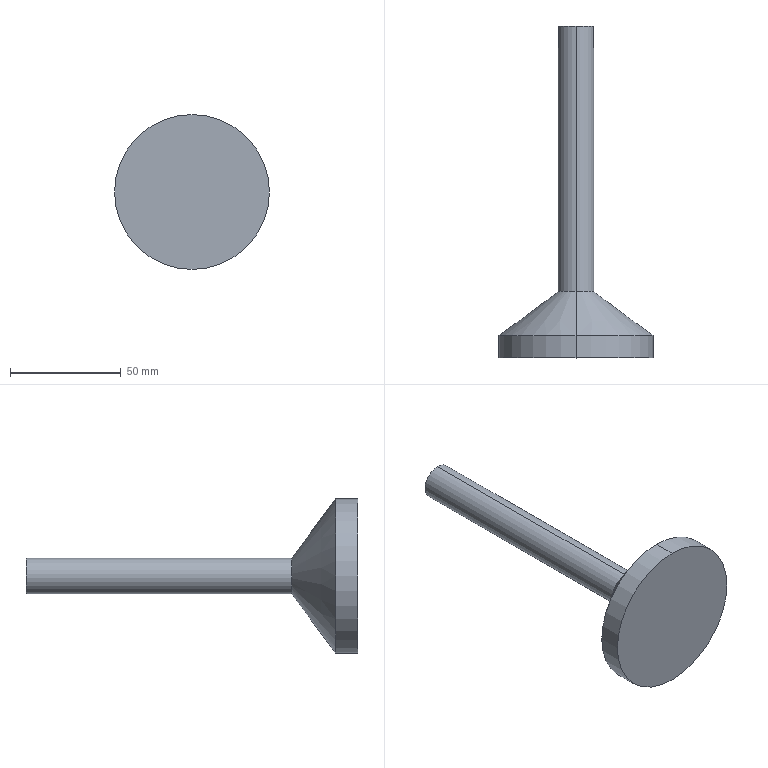Part | SolidWorks | features BaseBody 1 | 1 solid | 8 faces | box 70 x 150 x 70 mm | volume 95473 mm3 | cylinder 4 | cone 2 | plane 2 | commonest cylinder face diameters 16 x2 70 x2
STEP:
#1=CARTESIAN_POINT('',(0.,0.,-35.));
#2=VERTEX_POINT('',#1);
#3=CARTESIAN_POINT('',(0.,0.,35.));
#4=VERTEX_POINT('',#3);
#5=CARTESIAN_POINT('',(0.,0.,0.));
#6=DIRECTION('',(0.,-1.,0.));
#7=DIRECTION('',(0.,0.,1.));
#8=AXIS2_PLACEMENT_3D('',#5,#6,#7);
#9=CIRCLE('',#8,35.);
#10=EDGE_CURVE('',#2,#4,#9,.T.);
#11=ORIENTED_EDGE('',*,*,#10,.F.);
#12=CARTESIAN_POINT('',(0.,10.,-35.));
#13=VERTEX_POINT('',#12);
#14=CARTESIAN_POINT('',(0.,150.,-35.));
#15=DIRECTION('',(0.,1.,0.));
#16=VECTOR('',#15,1000.);
#17=LINE('',#14,#16);
#18=EDGE_CURVE('',#2,#13,#17,.T.);
#19=ORIENTED_EDGE('',*,*,#18,.T.);
#20=CARTESIAN_POINT('',(0.,10.,35.));
#21=VERTEX_POINT('',#20);
#22=CARTESIAN_POINT('',(0.,10.,0.));
#23=DIRECTION('',(0.,-1.,0.));
#24=DIRECTION('',(0.,0.,1.));
#25=AXIS2_PLACEMENT_3D('',#22,#23,#24);
#26=CIRCLE('',#25,35.);
#27=EDGE_CURVE('',#13,#21,#26,.T.);
#28=ORIENTED_EDGE('',*,*,#27,.T.);
#29=CARTESIAN_POINT('',(0.,150.,35.));
#30=DIRECTION('',(0.,1.,0.));
#31=VECTOR('',#30,1000.);
#32=LINE('',#29,#31);
#33=EDGE_CURVE('',#4,#21,#32,.T.);
#34=ORIENTED_EDGE('',*,*,#33,.F.);
#35=EDGE_LOOP('',(#11,#19,#28,#34));
#36=FACE_OUTER_BOUND('',#35,.T.);
#37=CARTESIAN_POINT('',(0.,150.,0.));
#38=DIRECTION('',(0.,1.,0.));
#39=DIRECTION('',(0.,0.,1.));
#40=AXIS2_PLACEMENT_3D('',#37,#38,#39);
#41=CYLINDRICAL_SURFACE('',#40,35.);
#42=ADVANCED_FACE('',(#36),#41,.T.);
#43=CARTESIAN_POINT('',(0.,30.,-8.));
#44=VERTEX_POINT('',#43);
#45=CARTESIAN_POINT('',(0.,30.,8.));
#46=VERTEX_POINT('',#45);
#47=CARTESIAN_POINT('',(0.,30.,0.));
#48=DIRECTION('',(0.,-1.,0.));
#49=DIRECTION('',(0.,0.,-1.));
#50=AXIS2_PLACEMENT_3D('',#47,#48,#49);
#51=CIRCLE('',#50,8.);
#52=EDGE_CURVE('',#44,#46,#51,.T.);
#53=ORIENTED_EDGE('',*,*,#52,.T.);
#54=CARTESIAN_POINT('',(0.,10.,35.));
#55=DIRECTION('',(0.,-0.5952,0.8036));
#56=VECTOR('',#55,1000.);
#57=LINE('',#54,#56);
#58=EDGE_CURVE('',#46,#21,#57,.T.);
#59=ORIENTED_EDGE('',*,*,#58,.T.);
#60=ORIENTED_EDGE('',*,*,#27,.F.);
#61=CARTESIAN_POINT('',(0.,10.,-35.));
#62=DIRECTION('',(0.,-0.5952,-0.8036));
#63=VECTOR('',#62,1000.);
#64=LINE('',#61,#63);
#65=EDGE_CURVE('',#44,#13,#64,.T.);
#66=ORIENTED_EDGE('',*,*,#65,.F.);
#67=EDGE_LOOP('',(#53,#59,#60,#66));
#68=FACE_OUTER_BOUND('',#67,.T.);
#69=CARTESIAN_POINT('',(0.,10.,0.));
#70=DIRECTION('',(0.,-1.,0.));
#71=DIRECTION('',(0.,0.,-1.));
#72=AXIS2_PLACEMENT_3D('',#69,#70,#71);
#73=CONICAL_SURFACE('',#72,35.,0.9332);
#74=ADVANCED_FACE('',(#68),#73,.T.);
#75=ORIENTED_EDGE('',*,*,#52,.F.);
#76=CARTESIAN_POINT('',(0.,150.,-8.));
#77=VERTEX_POINT('',#76);
#78=CARTESIAN_POINT('',(0.,150.,-8.));
#79=DIRECTION('',(0.,1.,0.));
#80=VECTOR('',#79,1000.);
#81=LINE('',#78,#80);
#82=EDGE_CURVE('',#44,#77,#81,.T.);
#83=ORIENTED_EDGE('',*,*,#82,.T.);
#84=CARTESIAN_POINT('',(0.,150.,8.));
#85=VERTEX_POINT('',#84);
#86=CARTESIAN_POINT('',(0.,150.,0.));
#87=DIRECTION('',(0.,-1.,0.));
#88=DIRECTION('',(0.,0.,1.));
#89=AXIS2_PLACEMENT_3D('',#86,#87,#88);
#90=CIRCLE('',#89,8.);
#91=EDGE_CURVE('',#77,#85,#90,.T.);
#92=ORIENTED_EDGE('',*,*,#91,.T.);
#93=CARTESIAN_POINT('',(0.,150.,8.));
#94=DIRECTION('',(0.,1.,0.));
#95=VECTOR('',#94,1000.);
#96=LINE('',#93,#95);
#97=EDGE_CURVE('',#46,#85,#96,.T.);
#98=ORIENTED_EDGE('',*,*,#97,.F.);
#99=EDGE_LOOP('',(#75,#83,#92,#98));
#100=FACE_OUTER_BOUND('',#99,.T.);
#101=CARTESIAN_POINT('',(0.,150.,0.));
#102=DIRECTION('',(0.,1.,0.));
#103=DIRECTION('',(0.,0.,1.));
#104=AXIS2_PLACEMENT_3D('',#101,#102,#103);
#105=CYLINDRICAL_SURFACE('',#104,8.);
#106=ADVANCED_FACE('',(#100),#105,.T.);
#107=CARTESIAN_POINT('',(0.,0.,0.));
#108=DIRECTION('',(0.,-1.,0.));
#109=DIRECTION('',(0.,0.,1.));
#110=AXIS2_PLACEMENT_3D('',#107,#108,#109);
#111=CIRCLE('',#110,35.);
#112=EDGE_CURVE('',#4,#2,#111,.T.);
#113=ORIENTED_EDGE('',*,*,#112,.T.);
#114=ORIENTED_EDGE('',*,*,#10,.T.);
#115=EDGE_LOOP('',(#113,#114));
#116=FACE_OUTER_BOUND('',#115,.T.);
#117=CARTESIAN_POINT('',(0.,0.,0.));
#118=DIRECTION('',(0.,-1.,0.));
#119=DIRECTION('',(0.,0.,-1.));
#120=AXIS2_PLACEMENT_3D('',#117,#118,#119);
#121=PLANE('',#120);
#122=ADVANCED_FACE('',(#116),#121,.T.);
#123=ORIENTED_EDGE('',*,*,#18,.F.);
#124=ORIENTED_EDGE('',*,*,#112,.F.);
#125=ORIENTED_EDGE('',*,*,#33,.T.);
#126=CARTESIAN_POINT('',(0.,10.,0.));
#127=DIRECTION('',(0.,-1.,0.));
#128=DIRECTION('',(0.,0.,1.));
#129=AXIS2_PLACEMENT_3D('',#126,#127,#128);
#130=CIRCLE('',#129,35.);
#131=EDGE_CURVE('',#21,#13,#130,.T.);
#132=ORIENTED_EDGE('',*,*,#131,.T.);
#133=EDGE_LOOP('',(#123,#124,#125,#132));
#134=FACE_OUTER_BOUND('',#133,.T.);
#135=CARTESIAN_POINT('',(0.,150.,0.));
#136=DIRECTION('',(0.,1.,0.));
#137=DIRECTION('',(0.,0.,1.));
#138=AXIS2_PLACEMENT_3D('',#135,#136,#137);
#139=CYLINDRICAL_SURFACE('',#138,35.);
#140=ADVANCED_FACE('',(#134),#139,.T.);
#141=ORIENTED_EDGE('',*,*,#58,.F.);
#142=CARTESIAN_POINT('',(0.,30.,0.));
#143=DIRECTION('',(0.,-1.,0.));
#144=DIRECTION('',(0.,0.,-1.));
#145=AXIS2_PLACEMENT_3D('',#142,#143,#144);
#146=CIRCLE('',#145,8.);
#147=EDGE_CURVE('',#46,#44,#146,.T.);
#148=ORIENTED_EDGE('',*,*,#147,.T.);
#149=ORIENTED_EDGE('',*,*,#65,.T.);
#150=ORIENTED_EDGE('',*,*,#131,.F.);
#151=EDGE_LOOP('',(#141,#148,#149,#150));
#152=FACE_OUTER_BOUND('',#151,.T.);
#153=CARTESIAN_POINT('',(0.,10.,0.));
#154=DIRECTION('',(0.,-1.,0.));
#155=DIRECTION('',(0.,0.,-1.));
#156=AXIS2_PLACEMENT_3D('',#153,#154,#155);
#157=CONICAL_SURFACE('',#156,35.,0.9332);
#158=ADVANCED_FACE('',(#152),#157,.T.);
#159=ORIENTED_EDGE('',*,*,#82,.F.);
#160=ORIENTED_EDGE('',*,*,#147,.F.);
#161=ORIENTED_EDGE('',*,*,#97,.T.);
#162=CARTESIAN_POINT('',(0.,150.,0.));
#163=DIRECTION('',(0.,-1.,0.));
#164=DIRECTION('',(0.,0.,1.));
#165=AXIS2_PLACEMENT_3D('',#162,#163,#164);
#166=CIRCLE('',#165,8.);
#167=EDGE_CURVE('',#85,#77,#166,.T.);
#168=ORIENTED_EDGE('',*,*,#167,.T.);
#169=EDGE_LOOP('',(#159,#160,#161,#168));
#170=FACE_OUTER_BOUND('',#169,.T.);
#171=CARTESIAN_POINT('',(0.,150.,0.));
#172=DIRECTION('',(0.,1.,0.));
#173=DIRECTION('',(0.,0.,1.));
#174=AXIS2_PLACEMENT_3D('',#171,#172,#173);
#175=CYLINDRICAL_SURFACE('',#174,8.);
#176=ADVANCED_FACE('',(#170),#175,.T.);
#177=ORIENTED_EDGE('',*,*,#167,.F.);
#178=ORIENTED_EDGE('',*,*,#91,.F.);
#179=EDGE_LOOP('',(#177,#178));
#180=FACE_OUTER_BOUND('',#179,.T.);
#181=CARTESIAN_POINT('',(0.,150.,8.));
#182=DIRECTION('',(0.,1.,0.));
#183=DIRECTION('',(0.,0.,1.));
#184=AXIS2_PLACEMENT_3D('',#181,#182,#183);
#185=PLANE('',#184);
#186=ADVANCED_FACE('',(#180),#185,.T.);
#187=CLOSED_SHELL('',(#42,#74,#106,#122,#140,#158,#176,#186));
#188=MANIFOLD_SOLID_BREP('',#187);
#189=CARTESIAN_POINT('',(0.,0.,0.));
#190=DIRECTION('',(0.,0.,1.));
#191=DIRECTION('',(1.,0.,0.));
#192=AXIS2_PLACEMENT_3D('',#189,#190,#191);
#193=(LENGTH_UNIT()NAMED_UNIT(*)SI_UNIT(.MILLI.,.METRE.));
#194=UNCERTAINTY_MEASURE_WITH_UNIT(LENGTH_MEASURE(0.00001),#193,'','');
#195=(NAMED_UNIT(*)PLANE_ANGLE_UNIT()SI_UNIT($,.RADIAN.));
#196=(NAMED_UNIT(*)SI_UNIT($,.STERADIAN.)SOLID_ANGLE_UNIT());
#197=(GEOMETRIC_REPRESENTATION_CONTEXT(3)GLOBAL_UNCERTAINTY_ASSIGNED_CONTEXT((#194))GLOBAL_UNIT_ASSIGNED_CONTEXT((#193,#195,#196))REPRESENTATION_CONTEXT('',''));
#198=ADVANCED_BREP_SHAPE_REPRESENTATION('',(#188,#192),#197);